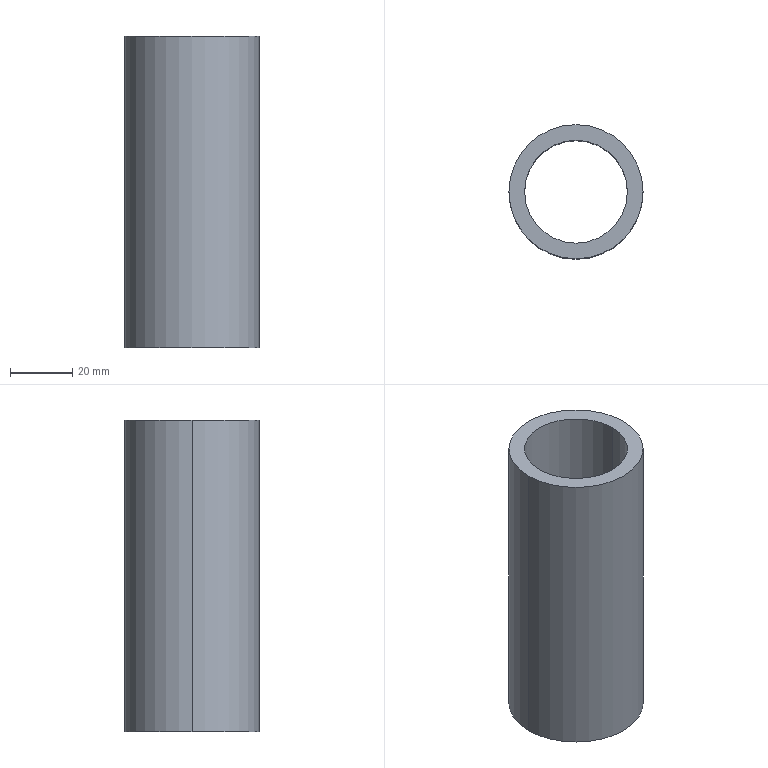Part | SolidWorks | features Extrusion 1 | 1 solid | 6 faces | box 43 x 43 x 100 mm | volume 59690 mm3 | cylinder 4 | plane 2 | commonest cylinder face diameters 33 x2 43 x2
STEP:
#1=CARTESIAN_POINT('',(-16.5,0.,100.));
#2=VERTEX_POINT('',#1);
#3=CARTESIAN_POINT('',(16.5,0.,100.));
#4=VERTEX_POINT('',#3);
#5=CARTESIAN_POINT('',(0.,0.,100.));
#6=DIRECTION('',(0.,0.,1.));
#7=DIRECTION('',(1.,0.,0.));
#8=AXIS2_PLACEMENT_3D('',#5,#6,#7);
#9=CIRCLE('',#8,16.5);
#10=EDGE_CURVE('',#2,#4,#9,.T.);
#11=ORIENTED_EDGE('',*,*,#10,.T.);
#12=CARTESIAN_POINT('',(16.5,0.,0.));
#13=VERTEX_POINT('',#12);
#14=CARTESIAN_POINT('',(16.5,0.,100.));
#15=DIRECTION('',(0.,0.,-1.));
#16=VECTOR('',#15,1000.);
#17=LINE('',#14,#16);
#18=EDGE_CURVE('',#4,#13,#17,.T.);
#19=ORIENTED_EDGE('',*,*,#18,.T.);
#20=CARTESIAN_POINT('',(-16.5,0.,0.));
#21=VERTEX_POINT('',#20);
#22=CARTESIAN_POINT('',(0.,0.,0.));
#23=DIRECTION('',(0.,0.,1.));
#24=DIRECTION('',(1.,0.,0.));
#25=AXIS2_PLACEMENT_3D('',#22,#23,#24);
#26=CIRCLE('',#25,16.5);
#27=EDGE_CURVE('',#21,#13,#26,.T.);
#28=ORIENTED_EDGE('',*,*,#27,.F.);
#29=CARTESIAN_POINT('',(-16.5,0.,100.));
#30=DIRECTION('',(0.,0.,-1.));
#31=VECTOR('',#30,1000.);
#32=LINE('',#29,#31);
#33=EDGE_CURVE('',#2,#21,#32,.T.);
#34=ORIENTED_EDGE('',*,*,#33,.F.);
#35=EDGE_LOOP('',(#11,#19,#28,#34));
#36=FACE_OUTER_BOUND('',#35,.T.);
#37=CARTESIAN_POINT('',(0.,0.,100.));
#38=DIRECTION('',(0.,0.,-1.));
#39=DIRECTION('',(-1.,0.,0.));
#40=AXIS2_PLACEMENT_3D('',#37,#38,#39);
#41=CYLINDRICAL_SURFACE('',#40,16.5);
#42=ADVANCED_FACE('',(#36),#41,.F.);
#43=CARTESIAN_POINT('',(21.5,0.,100.));
#44=VERTEX_POINT('',#43);
#45=CARTESIAN_POINT('',(-21.5,0.,100.));
#46=VERTEX_POINT('',#45);
#47=CARTESIAN_POINT('',(0.,0.,100.));
#48=DIRECTION('',(0.,0.,1.));
#49=DIRECTION('',(1.,0.,0.));
#50=AXIS2_PLACEMENT_3D('',#47,#48,#49);
#51=CIRCLE('',#50,21.5);
#52=EDGE_CURVE('',#44,#46,#51,.T.);
#53=ORIENTED_EDGE('',*,*,#52,.F.);
#54=CARTESIAN_POINT('',(21.5,0.,0.));
#55=VERTEX_POINT('',#54);
#56=CARTESIAN_POINT('',(21.5,0.,100.));
#57=DIRECTION('',(0.,0.,-1.));
#58=VECTOR('',#57,1000.);
#59=LINE('',#56,#58);
#60=EDGE_CURVE('',#44,#55,#59,.T.);
#61=ORIENTED_EDGE('',*,*,#60,.T.);
#62=CARTESIAN_POINT('',(-21.5,0.,0.));
#63=VERTEX_POINT('',#62);
#64=CARTESIAN_POINT('',(0.,0.,0.));
#65=DIRECTION('',(0.,0.,1.));
#66=DIRECTION('',(1.,0.,0.));
#67=AXIS2_PLACEMENT_3D('',#64,#65,#66);
#68=CIRCLE('',#67,21.5);
#69=EDGE_CURVE('',#55,#63,#68,.T.);
#70=ORIENTED_EDGE('',*,*,#69,.T.);
#71=CARTESIAN_POINT('',(-21.5,0.,100.));
#72=DIRECTION('',(0.,0.,-1.));
#73=VECTOR('',#72,1000.);
#74=LINE('',#71,#73);
#75=EDGE_CURVE('',#46,#63,#74,.T.);
#76=ORIENTED_EDGE('',*,*,#75,.F.);
#77=EDGE_LOOP('',(#53,#61,#70,#76));
#78=FACE_OUTER_BOUND('',#77,.T.);
#79=CARTESIAN_POINT('',(0.,0.,100.));
#80=DIRECTION('',(0.,0.,-1.));
#81=DIRECTION('',(-1.,0.,0.));
#82=AXIS2_PLACEMENT_3D('',#79,#80,#81);
#83=CYLINDRICAL_SURFACE('',#82,21.5);
#84=ADVANCED_FACE('',(#78),#83,.T.);
#85=CARTESIAN_POINT('',(0.,0.,100.));
#86=DIRECTION('',(0.,0.,1.));
#87=DIRECTION('',(1.,0.,0.));
#88=AXIS2_PLACEMENT_3D('',#85,#86,#87);
#89=CIRCLE('',#88,21.5);
#90=EDGE_CURVE('',#46,#44,#89,.T.);
#91=ORIENTED_EDGE('',*,*,#90,.T.);
#92=ORIENTED_EDGE('',*,*,#52,.T.);
#93=EDGE_LOOP('',(#91,#92));
#94=FACE_OUTER_BOUND('',#93,.T.);
#95=ORIENTED_EDGE('',*,*,#10,.F.);
#96=CARTESIAN_POINT('',(0.,0.,100.));
#97=DIRECTION('',(0.,0.,1.));
#98=DIRECTION('',(1.,0.,0.));
#99=AXIS2_PLACEMENT_3D('',#96,#97,#98);
#100=CIRCLE('',#99,16.5);
#101=EDGE_CURVE('',#4,#2,#100,.T.);
#102=ORIENTED_EDGE('',*,*,#101,.F.);
#103=EDGE_LOOP('',(#95,#102));
#104=FACE_BOUND('',#103,.T.);
#105=CARTESIAN_POINT('',(0.,0.,100.));
#106=DIRECTION('',(0.,0.,1.));
#107=DIRECTION('',(1.,0.,0.));
#108=AXIS2_PLACEMENT_3D('',#105,#106,#107);
#109=PLANE('',#108);
#110=ADVANCED_FACE('',(#94,#104),#109,.T.);
#111=CARTESIAN_POINT('',(0.,0.,0.));
#112=DIRECTION('',(0.,0.,1.));
#113=DIRECTION('',(1.,0.,0.));
#114=AXIS2_PLACEMENT_3D('',#111,#112,#113);
#115=CIRCLE('',#114,21.5);
#116=EDGE_CURVE('',#63,#55,#115,.T.);
#117=ORIENTED_EDGE('',*,*,#116,.F.);
#118=ORIENTED_EDGE('',*,*,#69,.F.);
#119=EDGE_LOOP('',(#117,#118));
#120=FACE_OUTER_BOUND('',#119,.T.);
#121=ORIENTED_EDGE('',*,*,#27,.T.);
#122=CARTESIAN_POINT('',(0.,0.,0.));
#123=DIRECTION('',(0.,0.,1.));
#124=DIRECTION('',(1.,0.,0.));
#125=AXIS2_PLACEMENT_3D('',#122,#123,#124);
#126=CIRCLE('',#125,16.5);
#127=EDGE_CURVE('',#13,#21,#126,.T.);
#128=ORIENTED_EDGE('',*,*,#127,.T.);
#129=EDGE_LOOP('',(#121,#128));
#130=FACE_BOUND('',#129,.T.);
#131=CARTESIAN_POINT('',(0.,0.,0.));
#132=DIRECTION('',(0.,0.,1.));
#133=DIRECTION('',(1.,0.,0.));
#134=AXIS2_PLACEMENT_3D('',#131,#132,#133);
#135=PLANE('',#134);
#136=ADVANCED_FACE('',(#120,#130),#135,.F.);
#137=ORIENTED_EDGE('',*,*,#60,.F.);
#138=ORIENTED_EDGE('',*,*,#90,.F.);
#139=ORIENTED_EDGE('',*,*,#75,.T.);
#140=ORIENTED_EDGE('',*,*,#116,.T.);
#141=EDGE_LOOP('',(#137,#138,#139,#140));
#142=FACE_OUTER_BOUND('',#141,.T.);
#143=CARTESIAN_POINT('',(0.,0.,100.));
#144=DIRECTION('',(0.,0.,-1.));
#145=DIRECTION('',(-1.,0.,0.));
#146=AXIS2_PLACEMENT_3D('',#143,#144,#145);
#147=CYLINDRICAL_SURFACE('',#146,21.5);
#148=ADVANCED_FACE('',(#142),#147,.T.);
#149=ORIENTED_EDGE('',*,*,#18,.F.);
#150=ORIENTED_EDGE('',*,*,#101,.T.);
#151=ORIENTED_EDGE('',*,*,#33,.T.);
#152=ORIENTED_EDGE('',*,*,#127,.F.);
#153=EDGE_LOOP('',(#149,#150,#151,#152));
#154=FACE_OUTER_BOUND('',#153,.T.);
#155=CARTESIAN_POINT('',(0.,0.,100.));
#156=DIRECTION('',(0.,0.,-1.));
#157=DIRECTION('',(-1.,0.,0.));
#158=AXIS2_PLACEMENT_3D('',#155,#156,#157);
#159=CYLINDRICAL_SURFACE('',#158,16.5);
#160=ADVANCED_FACE('',(#154),#159,.F.);
#161=CLOSED_SHELL('',(#42,#84,#110,#136,#148,#160));
#162=MANIFOLD_SOLID_BREP('',#161);
#163=CARTESIAN_POINT('',(0.,0.,0.));
#164=DIRECTION('',(0.,0.,1.));
#165=DIRECTION('',(1.,0.,0.));
#166=AXIS2_PLACEMENT_3D('',#163,#164,#165);
#167=(LENGTH_UNIT()NAMED_UNIT(*)SI_UNIT(.MILLI.,.METRE.));
#168=UNCERTAINTY_MEASURE_WITH_UNIT(LENGTH_MEASURE(0.00001),#167,'','');
#169=(NAMED_UNIT(*)PLANE_ANGLE_UNIT()SI_UNIT($,.RADIAN.));
#170=(NAMED_UNIT(*)SI_UNIT($,.STERADIAN.)SOLID_ANGLE_UNIT());
#171=(GEOMETRIC_REPRESENTATION_CONTEXT(3)GLOBAL_UNCERTAINTY_ASSIGNED_CONTEXT((#168))GLOBAL_UNIT_ASSIGNED_CONTEXT((#167,#169,#170))REPRESENTATION_CONTEXT('',''));
#172=ADVANCED_BREP_SHAPE_REPRESENTATION('',(#162,#166),#171);